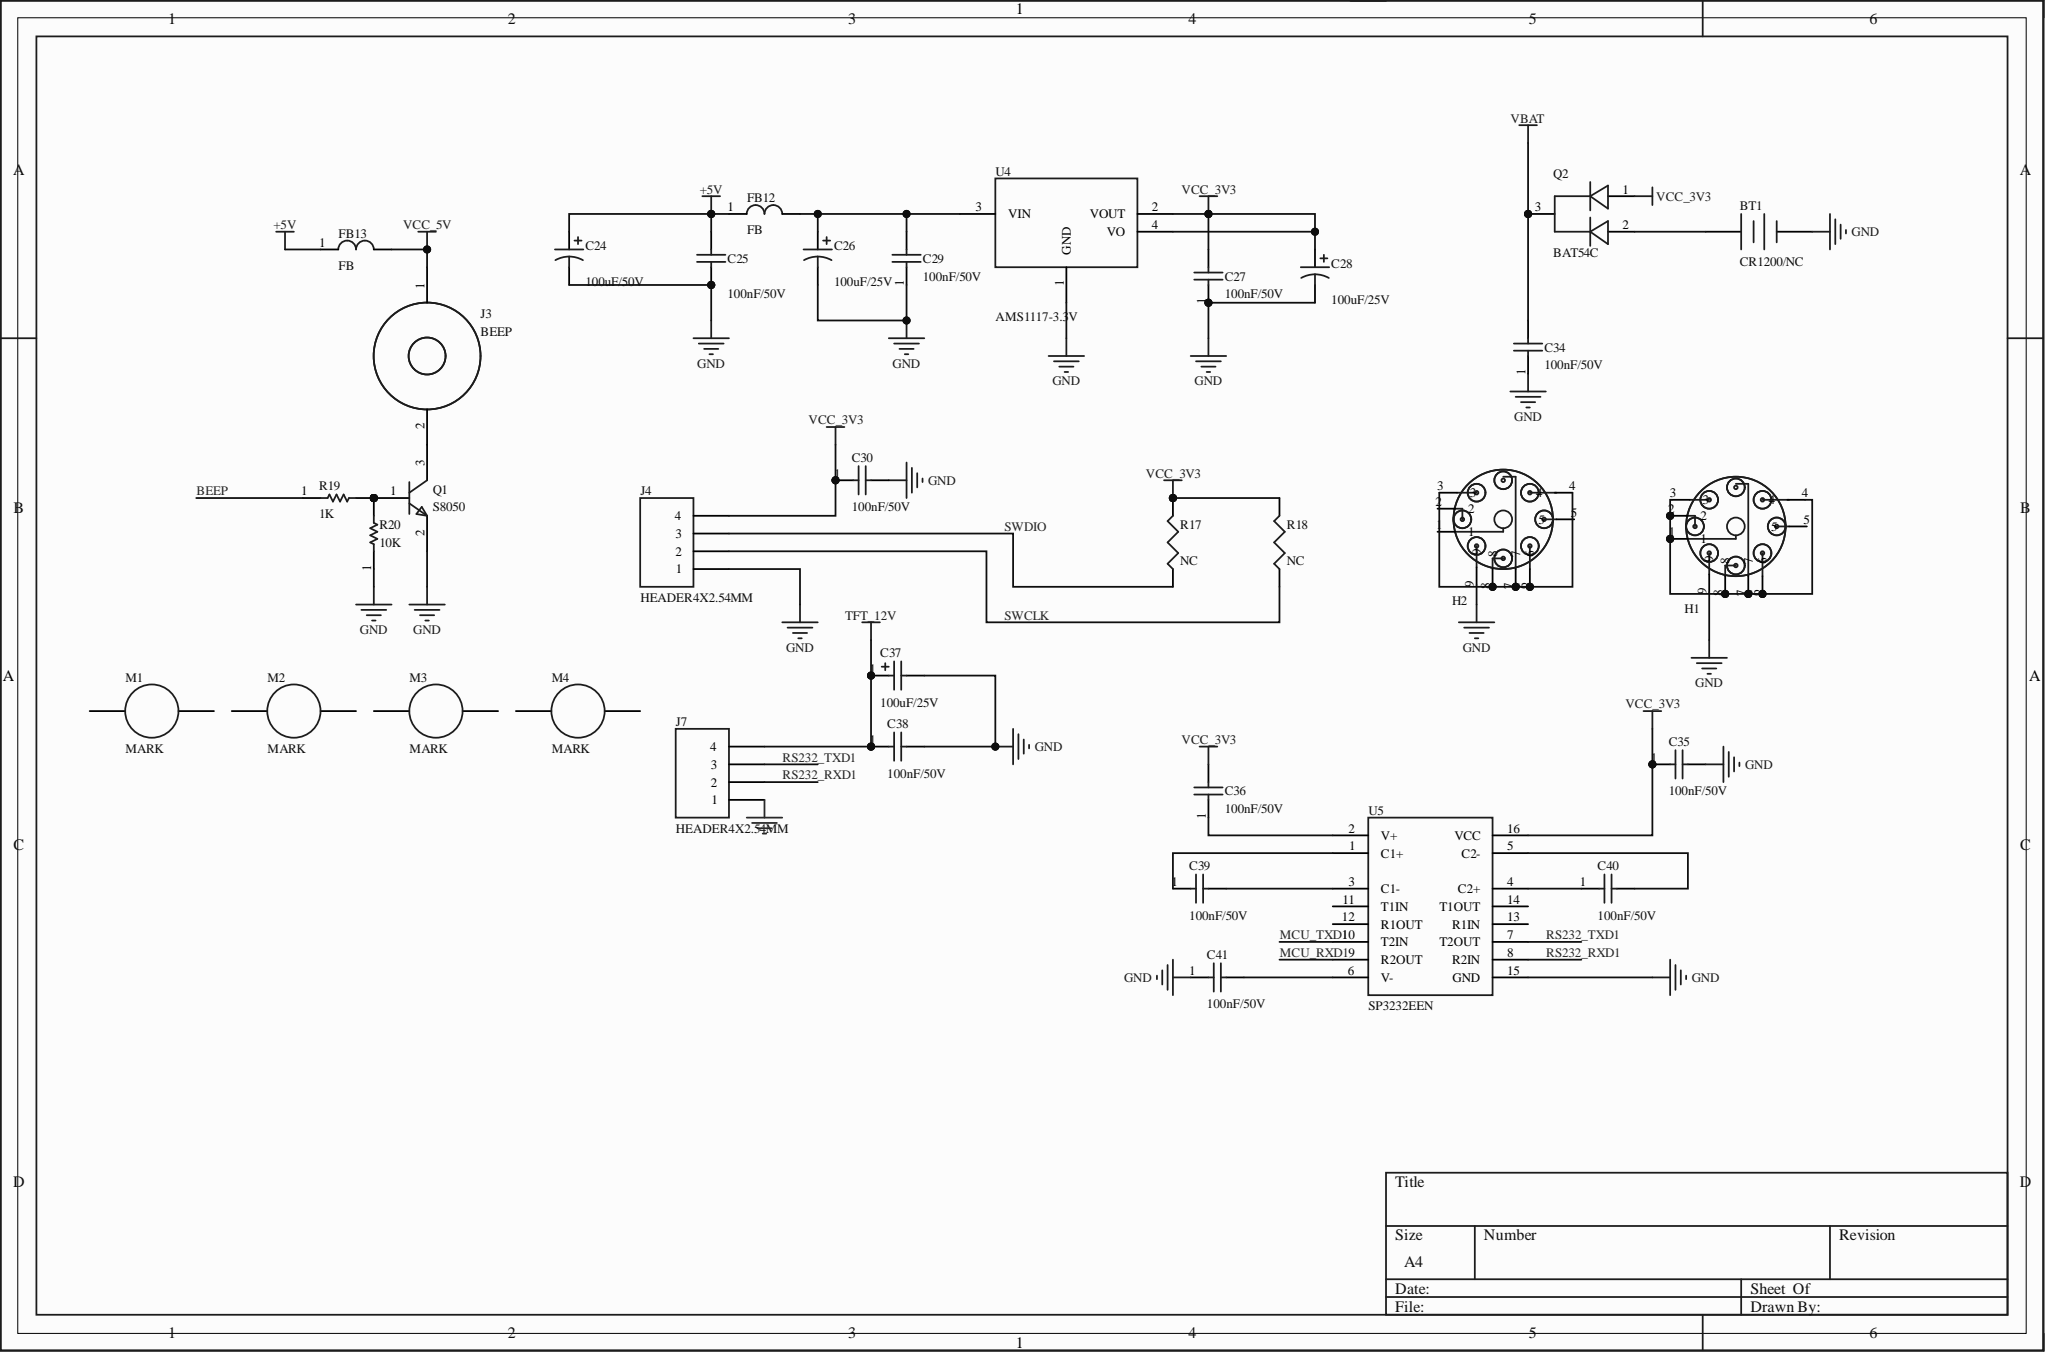Circuit board | Altium Designer | 35 parts | 22 nets
Bill of materials:
Comment,Description,Designator,Footprint,LibRef,Quantity
"CR1200/NC","Multicell Battery","BT1","BAT-2","CR1200/NC","1"
"","Polarized Capacitor (Surface Mount)","C24, C26, C28","C0805","Cap Pol3","3"
"","Capacitor","C25","RAD-0.3","Cap","1"
"Cap","Capacitor","C27, C29, C30, C34, C35, C36, C38, C39, C40, C41","0603_C","Cap","10"
"Cap Pol1","Polarized Capacitor (Radial)","C37","CAP-SMD_BD6.3-L6.6-W6.6-FD","Cap Pol1","1"
"FB","","FB12, FB13","0603_L","FB","2"
"H","","H1, H2","HOLE-ZR","H","2"
"BEEP","","J3","BUZ-TH_BD12.0-P7.60-D0.6-FD","BEEP","1"
"HEADER4X2.54MM","Header, 4-Pin","J4, J7","CN4$2F$DIP$2F$P2.54B","HEADER4X2.54MM","2"
"MARK","Indicating Instrument","M1, M2, M3, M4","RAD-0.1","MARK","4"
"S8050","NPN Bipolar Transistor","Q1","SOT-23(SOT-23-3)","S8050","1"
"BAT54C","","Q2","SOT-23(SOT-23-3)","BAT54C","1"
"","Resistor","R17, R18","J1-0603","Res3","2"
"1K","Resistor","R19","0603_R","1K","1"
"10K","Resistor","R20","0603_R","10K","1"
"AMS1117-3.3V","","U4","SOT-223","AMS1117-3.3V","1"
"SP3232EEN","","U5","SOP-16_150MIL","SP3232EEN","1"
Netlist (Protel format):
[
BT1
BAT-2
CR1200/NC



]
[
C24
C0805




]
[
C25
RAD-0.3




]
[
C26
C0805




]
[
C27
0603_C
Cap



]
[
C28
C0805




]
[
C29
0603_C
Cap



]
[
C30
0603_C
Cap



]
[
C34
0603_C
Cap



]
[
C35
0603_C
Cap



]
[
C36
0603_C
Cap



]
[
C37
CAP-SMD_BD6.3-L6.6-W6.6-FD
Cap Pol1



]
[
C38
0603_C
Cap



]
[
C39
0603_C
Cap



]
[
C40
0603_C
Cap



]
[
C41
0603_C
Cap



]
[
FB12
0603_L
FB



]
[
FB13
0603_L
FB



]
[
H1
HOLE-ZR
H



]
[
H2
HOLE-ZR
H



]
[
J3
BUZ-TH_BD12.0-P7.60-D0.6-FD
BEEP



]
[
J4
CN4$2F$DIP$2F$P2.54B
HEADER4X2.54MM



]
[
J7
CN4$2F$DIP$2F$P2.54B
HEADER4X2.54MM



]
[
M1
RAD-0.1
MARK



]
[
M2
RAD-0.1
MARK



]
[
M3
RAD-0.1
MARK



]
[
M4
RAD-0.1
MARK



]
[
Q1
SOT-23(SOT-23-3)
S8050



]
[
Q2
SOT-23(SOT-23-3)
BAT54C



]
[
R17
J1-0603




]
[
R18
J1-0603




]
[
R19
0603_R
1K



]
[
R20
0603_R
10K



]
[
U4
SOT-223
AMS1117-3.3V



]
[
U5
SOP-16_150MIL
SP3232EEN



]
(
VCC_5V
FB13-2
J3-1
)
(
VCC_3V3
C27-2
C28-1
C30-1
C35-1
C36-2
J4-4
Q2-1
R17-2
R18-2
U4-2
U4-4
U5-16
)
(
VBAT
C34-2
Q2-3
)
(
TFT_12V
C37-1
C38-1
J7-4
)
(
SWDIO
J4-3
R17-1
)
(
SWCLK
J4-2
R18-1
)
(
RS232_TXD1
J7-3
U5-7
)
(
RS232_RXD1
J7-2
U5-8
)
(
NetQ1_1
Q1-1
R19-2
R20-2
)
(
NetJ3_2
J3-2
Q1-3
)
(
NetH2_3
H2-3
H2-4
H2-6
H2-7
H2-8
)
(
NetH1_1
H1-1
H1-2
H1-3
H1-4
H1-6
H1-7
H1-8
)
(
NetC41_2
C41-2
U5-6
)
(
NetC40_2
C40-2
U5-5
)
(
NetC40_1
C40-1
U5-4
)
(
NetC39_2
C39-2
U5-3
)
(
NetC39_1
C39-1
U5-1
)
(
NetC36_1
C36-1
U5-2
)
(
NetC26_1
C26-1
C29-2
FB12-2
U4-3
)
(
NetBT1_1
BT1-1
Q2-2
)
(
GND
BT1-2
C24-2
C25-1
C26-2
C27-1
C28-2
C29-1
C30-2
C34-1
C35-2
C37-2
C38-2
C41-1
H1-9
H2-9
J4-1
J7-1
Q1-2
R20-1
U4-1
U5-15
)
(
+5V
C24-1
C25-2
FB12-1
FB13-1
)